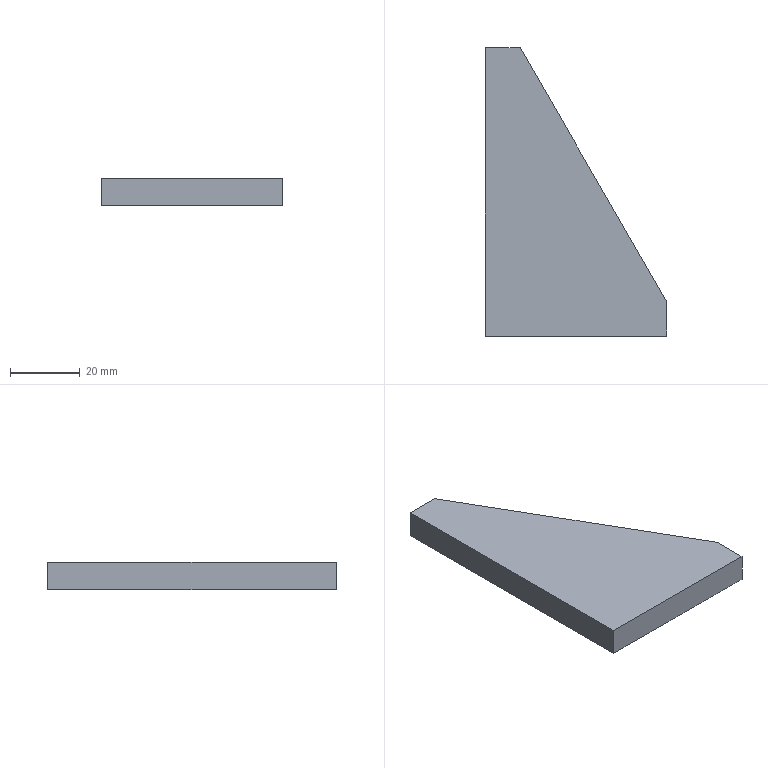Part | STEP file | X77-03213 | 1 solid | 7 faces | box 52 x 82.746 x 8 mm | volume 22201 mm3 | plane 7
STEP:
#1=CARTESIAN_POINT('',(20.,9.91,0.));
#2=VERTEX_POINT('',#1);
#3=CARTESIAN_POINT('',(10.,9.91,0.));
#4=VERTEX_POINT('',#3);
#5=CARTESIAN_POINT('',(10.,9.91,0.));
#6=DIRECTION('',(-1.,0.,0.));
#7=VECTOR('',#6,1000.);
#8=LINE('',#5,#7);
#9=EDGE_CURVE('',#2,#4,#8,.T.);
#10=ORIENTED_EDGE('',*,*,#9,.T.);
#11=CARTESIAN_POINT('',(10.,9.91,8.));
#12=VERTEX_POINT('',#11);
#13=CARTESIAN_POINT('',(10.,9.91,8.));
#14=DIRECTION('',(0.,0.,-1.));
#15=VECTOR('',#14,1000.);
#16=LINE('',#13,#15);
#17=EDGE_CURVE('',#12,#4,#16,.T.);
#18=ORIENTED_EDGE('',*,*,#17,.F.);
#19=CARTESIAN_POINT('',(20.,9.91,8.));
#20=VERTEX_POINT('',#19);
#21=CARTESIAN_POINT('',(10.,9.91,8.));
#22=DIRECTION('',(-1.,0.,0.));
#23=VECTOR('',#22,1000.);
#24=LINE('',#21,#23);
#25=EDGE_CURVE('',#20,#12,#24,.T.);
#26=ORIENTED_EDGE('',*,*,#25,.F.);
#27=CARTESIAN_POINT('',(20.,9.91,8.));
#28=DIRECTION('',(0.,0.,-1.));
#29=VECTOR('',#28,1000.);
#30=LINE('',#27,#29);
#31=EDGE_CURVE('',#20,#2,#30,.T.);
#32=ORIENTED_EDGE('',*,*,#31,.T.);
#33=EDGE_LOOP('',(#10,#18,#26,#32));
#34=FACE_OUTER_BOUND('',#33,.T.);
#35=CARTESIAN_POINT('',(10.,9.91,8.));
#36=DIRECTION('',(0.,-1.,0.));
#37=DIRECTION('',(0.,0.,-1.));
#38=AXIS2_PLACEMENT_3D('',#35,#36,#37);
#39=PLANE('',#38);
#40=ADVANCED_FACE('',(#34),#39,.F.);
#41=CARTESIAN_POINT('',(10.,-72.836,0.));
#42=VERTEX_POINT('',#41);
#43=CARTESIAN_POINT('',(10.,-72.836,0.));
#44=DIRECTION('',(0.,-1.,0.));
#45=VECTOR('',#44,1000.);
#46=LINE('',#43,#45);
#47=EDGE_CURVE('',#4,#42,#46,.T.);
#48=ORIENTED_EDGE('',*,*,#47,.T.);
#49=CARTESIAN_POINT('',(10.,-72.836,8.));
#50=VERTEX_POINT('',#49);
#51=CARTESIAN_POINT('',(10.,-72.836,8.));
#52=DIRECTION('',(0.,0.,-1.));
#53=VECTOR('',#52,1000.);
#54=LINE('',#51,#53);
#55=EDGE_CURVE('',#50,#42,#54,.T.);
#56=ORIENTED_EDGE('',*,*,#55,.F.);
#57=CARTESIAN_POINT('',(10.,-72.836,8.));
#58=DIRECTION('',(0.,-1.,0.));
#59=VECTOR('',#58,1000.);
#60=LINE('',#57,#59);
#61=EDGE_CURVE('',#12,#50,#60,.T.);
#62=ORIENTED_EDGE('',*,*,#61,.F.);
#63=ORIENTED_EDGE('',*,*,#17,.T.);
#64=EDGE_LOOP('',(#48,#56,#62,#63));
#65=FACE_OUTER_BOUND('',#64,.T.);
#66=CARTESIAN_POINT('',(10.,-72.836,8.));
#67=DIRECTION('',(1.,0.,0.));
#68=DIRECTION('',(0.,1.,0.));
#69=AXIS2_PLACEMENT_3D('',#66,#67,#68);
#70=PLANE('',#69);
#71=ADVANCED_FACE('',(#65),#70,.F.);
#72=CARTESIAN_POINT('',(62.,-72.836,0.));
#73=VERTEX_POINT('',#72);
#74=CARTESIAN_POINT('',(62.,-72.836,0.));
#75=DIRECTION('',(1.,0.,0.));
#76=VECTOR('',#75,1000.);
#77=LINE('',#74,#76);
#78=EDGE_CURVE('',#42,#73,#77,.T.);
#79=ORIENTED_EDGE('',*,*,#78,.T.);
#80=CARTESIAN_POINT('',(62.,-72.836,8.));
#81=VERTEX_POINT('',#80);
#82=CARTESIAN_POINT('',(62.,-72.836,8.));
#83=DIRECTION('',(0.,0.,-1.));
#84=VECTOR('',#83,1000.);
#85=LINE('',#82,#84);
#86=EDGE_CURVE('',#81,#73,#85,.T.);
#87=ORIENTED_EDGE('',*,*,#86,.F.);
#88=CARTESIAN_POINT('',(62.,-72.836,8.));
#89=DIRECTION('',(1.,0.,0.));
#90=VECTOR('',#89,1000.);
#91=LINE('',#88,#90);
#92=EDGE_CURVE('',#50,#81,#91,.T.);
#93=ORIENTED_EDGE('',*,*,#92,.F.);
#94=ORIENTED_EDGE('',*,*,#55,.T.);
#95=EDGE_LOOP('',(#79,#87,#93,#94));
#96=FACE_OUTER_BOUND('',#95,.T.);
#97=CARTESIAN_POINT('',(62.,-72.836,8.));
#98=DIRECTION('',(0.,1.,0.));
#99=DIRECTION('',(-1.,0.,0.));
#100=AXIS2_PLACEMENT_3D('',#97,#98,#99);
#101=PLANE('',#100);
#102=ADVANCED_FACE('',(#96),#101,.F.);
#103=CARTESIAN_POINT('',(62.,-62.836,0.));
#104=VERTEX_POINT('',#103);
#105=CARTESIAN_POINT('',(62.,-62.836,0.));
#106=DIRECTION('',(0.,1.,0.));
#107=VECTOR('',#106,1000.);
#108=LINE('',#105,#107);
#109=EDGE_CURVE('',#73,#104,#108,.T.);
#110=ORIENTED_EDGE('',*,*,#109,.T.);
#111=CARTESIAN_POINT('',(62.,-62.836,8.));
#112=VERTEX_POINT('',#111);
#113=CARTESIAN_POINT('',(62.,-62.836,8.));
#114=DIRECTION('',(0.,0.,-1.));
#115=VECTOR('',#114,1000.);
#116=LINE('',#113,#115);
#117=EDGE_CURVE('',#112,#104,#116,.T.);
#118=ORIENTED_EDGE('',*,*,#117,.F.);
#119=CARTESIAN_POINT('',(62.,-62.836,8.));
#120=DIRECTION('',(0.,1.,0.));
#121=VECTOR('',#120,1000.);
#122=LINE('',#119,#121);
#123=EDGE_CURVE('',#81,#112,#122,.T.);
#124=ORIENTED_EDGE('',*,*,#123,.F.);
#125=ORIENTED_EDGE('',*,*,#86,.T.);
#126=EDGE_LOOP('',(#110,#118,#124,#125));
#127=FACE_OUTER_BOUND('',#126,.T.);
#128=CARTESIAN_POINT('',(62.,-62.836,8.));
#129=DIRECTION('',(-1.,0.,0.));
#130=DIRECTION('',(0.,0.,1.));
#131=AXIS2_PLACEMENT_3D('',#128,#129,#130);
#132=PLANE('',#131);
#133=ADVANCED_FACE('',(#127),#132,.F.);
#134=CARTESIAN_POINT('',(20.,9.91,0.));
#135=DIRECTION('',(-0.5,0.866,0.));
#136=VECTOR('',#135,1000.);
#137=LINE('',#134,#136);
#138=EDGE_CURVE('',#104,#2,#137,.T.);
#139=ORIENTED_EDGE('',*,*,#138,.T.);
#140=ORIENTED_EDGE('',*,*,#31,.F.);
#141=CARTESIAN_POINT('',(20.,9.91,8.));
#142=DIRECTION('',(-0.5,0.866,0.));
#143=VECTOR('',#142,1000.);
#144=LINE('',#141,#143);
#145=EDGE_CURVE('',#112,#20,#144,.T.);
#146=ORIENTED_EDGE('',*,*,#145,.F.);
#147=ORIENTED_EDGE('',*,*,#117,.T.);
#148=EDGE_LOOP('',(#139,#140,#146,#147));
#149=FACE_OUTER_BOUND('',#148,.T.);
#150=CARTESIAN_POINT('',(20.,9.91,8.));
#151=DIRECTION('',(-0.866,-0.5,0.));
#152=DIRECTION('',(0.5,-0.866,0.));
#153=AXIS2_PLACEMENT_3D('',#150,#151,#152);
#154=PLANE('',#153);
#155=ADVANCED_FACE('',(#149),#154,.F.);
#156=ORIENTED_EDGE('',*,*,#25,.T.);
#157=ORIENTED_EDGE('',*,*,#61,.T.);
#158=ORIENTED_EDGE('',*,*,#92,.T.);
#159=ORIENTED_EDGE('',*,*,#123,.T.);
#160=ORIENTED_EDGE('',*,*,#145,.T.);
#161=EDGE_LOOP('',(#156,#157,#158,#159,#160));
#162=FACE_OUTER_BOUND('',#161,.T.);
#163=CARTESIAN_POINT('',(62.,9.91,8.));
#164=DIRECTION('',(0.,0.,-1.));
#165=DIRECTION('',(-1.,0.,0.));
#166=AXIS2_PLACEMENT_3D('',#163,#164,#165);
#167=PLANE('',#166);
#168=ADVANCED_FACE('',(#162),#167,.F.);
#169=ORIENTED_EDGE('',*,*,#9,.F.);
#170=ORIENTED_EDGE('',*,*,#138,.F.);
#171=ORIENTED_EDGE('',*,*,#109,.F.);
#172=ORIENTED_EDGE('',*,*,#78,.F.);
#173=ORIENTED_EDGE('',*,*,#47,.F.);
#174=EDGE_LOOP('',(#169,#170,#171,#172,#173));
#175=FACE_OUTER_BOUND('',#174,.T.);
#176=CARTESIAN_POINT('',(62.,9.91,0.));
#177=DIRECTION('',(0.,0.,-1.));
#178=DIRECTION('',(-1.,0.,0.));
#179=AXIS2_PLACEMENT_3D('',#176,#177,#178);
#180=PLANE('',#179);
#181=ADVANCED_FACE('',(#175),#180,.T.);
#182=CLOSED_SHELL('',(#40,#71,#102,#133,#155,#168,#181));
#183=MANIFOLD_SOLID_BREP('',#182);
#184=CARTESIAN_POINT('',(0.,0.,0.));
#185=DIRECTION('',(0.,0.,1.));
#186=DIRECTION('',(1.,0.,0.));
#187=AXIS2_PLACEMENT_3D('',#184,#185,#186);
#188=(LENGTH_UNIT()NAMED_UNIT(*)SI_UNIT(.MILLI.,.METRE.));
#189=UNCERTAINTY_MEASURE_WITH_UNIT(LENGTH_MEASURE(0.00001),#188,'','');
#190=(NAMED_UNIT(*)PLANE_ANGLE_UNIT()SI_UNIT($,.RADIAN.));
#191=(NAMED_UNIT(*)SI_UNIT($,.STERADIAN.)SOLID_ANGLE_UNIT());
#192=(GEOMETRIC_REPRESENTATION_CONTEXT(3)GLOBAL_UNCERTAINTY_ASSIGNED_CONTEXT((#189))GLOBAL_UNIT_ASSIGNED_CONTEXT((#188,#190,#191))REPRESENTATION_CONTEXT('',''));
#193=ADVANCED_BREP_SHAPE_REPRESENTATION('',(#183,#187),#192);